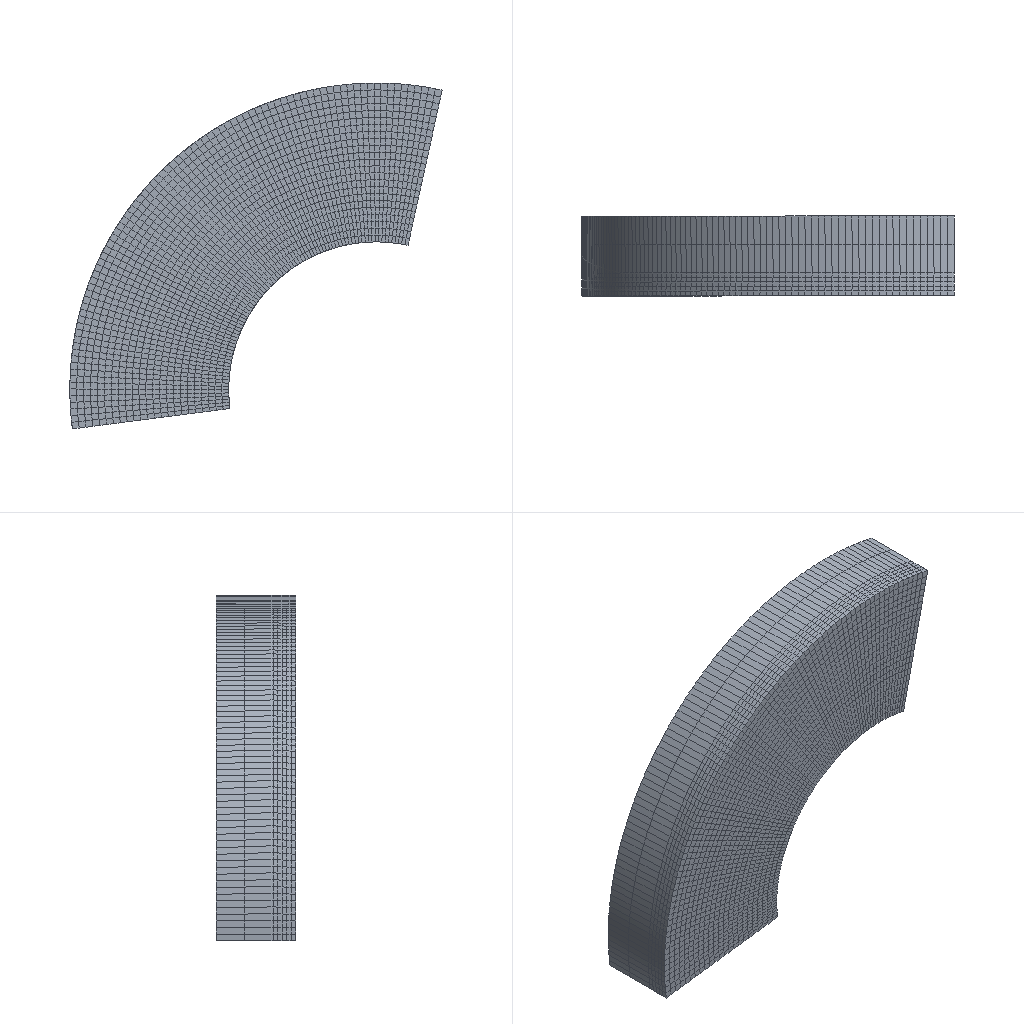Simulation study | abaqus
Set-up summary:
category,name,step,type,value,unit,region
solver,abaqus
solver,version,,,Abaqus/Explicit 2020
units,not stated in the deck,,not stated
analysis,deck,,transient,transient
load_step,Step-1,Step-1,transient,nlgeom=True
contact,interactions,,,general=0 pairs=1 ties=0
load_step,requested,,,1
mesh,nodes,,,17698
mesh,elements,,,14845
element_type,R3D3,,rigid,14
element_type,R3D4,,rigid,985
element_type,C3D8R,,solid,13846
load,load commands in deck,,count,1
bc,support commands in deck,,count,7
material,MATERIAL-1,,in results
check,setup vs results,,match,"per instance, exact: element labels, types and connectivity; labels of the nodes the elements use; coordinates of those nodes at SINGLE_PRECISION in 1 of 2 instance(s)"
Abaqus input file, long lists of numbers shortened:
*Heading
** Job name: Job-2 Model name: Model-1-Copy
** Generated by: Abaqus/CAE 2020
*Preprint, echo=NO, model=NO, history=NO, contact=NO
**
** PARTS
**
*Part, name=work
*Node
      1,  0.8032,          -5.,  -4.555
      2,  0.5209,  0.04385,  -2.954
** (992 more lines like these left out)
*Element, type=R3D4
1,   1,  15, 228,  19
2,  15,   2,   3, 228
** (983 more lines like these left out)
*Element, type=R3D3
77, 415, 376, 414
78, 365, 364, 321
** (12 more lines like these left out)
*End Part
**
*Part, name=work2
*Node
      1,   29.301,   24.684,          10.
      2,  -36.312,   49.078,          10.
** (16702 more lines like these left out)
*Element, type=C3D8R
   1,    1,   17,  675,  230,  444, 4585, 7355, 4415
   2,   17,   18,  676,  675, 4585, 4586, 7356, 7355
** (13844 more lines like these left out)
*Nset, nset=Set-1, generate
     1,  16704,      1
*Elset, elset=Set-1, generate
     1,  13846,      1
** Section: bing
*Solid Section, elset=Set-1, material=Material-1
,
*End Part
**
**
** ASSEMBLY
**
*Assembly, name=Assembly
**
*Instance, name=work-1, part=work
-40.107,           5., -16.132
-40.107,           5., -16.132, -40.126, 5.142, -17.122, 15.357
*End Instance
**
*Instance, name=work2-1, part=work2
0.00232,           0., 20.53
0.00232,           0., 20.53, -0.9849, 0.1125, 20.643, 90.734
*End Instance
**
*Node
      1,   87.459,          10.,  -1.747
*Nset, nset=Set-3, instance=work2-1
    5,    6,    7,    8,    9,   10,  231,  232,  233,  234,  235,  236,  237,  238,  239,  240
  241,  242,  243,  244,  245,  246,  247,  248,  249,  250,  251,  252,  253,  254,  255,  256
** (129 more lines like these left out)
*Elset, elset=Set-3, instance=work2-1, generate
 1979,  3956,     1
*Nset, nset=Set-7
 1,
*Nset, nset=b_Set-5, instance=work-1, generate
   1,  994,    1
*Elset, elset=b_Set-5, instance=work-1, generate
   1,  999,    1
*Nset, nset=s_Set-4, instance=work2-1
    1,    2,    3,    4,   11,   12,   13,   14,   15,   16,   17,   18,   19,   20,   21,   22
   23,   24,   25,   26,   27,   28,   29,   30,   31,   32,   33,   34,   35,   36,   37,   38
** (197 more lines like these left out)
*Elset, elset=s_Set-4, instance=work2-1
  3957,  3958,  3959,  3960,  3961,  3962,  3963,  3964,  3965,  3966,  3967,  3968,  3969,  3970,  3971,  3972
  3973,  3974,  3975,  3976,  3977,  3978,  3979,  3980,  3981,  3982,  3983,  3984,  3985,  3986,  3987,  3988
** (176 more lines like these left out)
*Nset, nset=s_Set-6, instance=work2-1
     1,     2,     3,     4,    11,    12,    13,    14,    15,    16,    17,    18,    19,    20,    21,    22
    23,    24,    25,    26,    27,    28,    29,    30,    31,    32,    33,    34,    35,    36,    37,    38
** (781 more lines like these left out)
*Elset, elset=s_Set-6, instance=work2-1, generate
  3957,  13846,      1
*Nset, nset=_PickedSet8, internal
 1,
*Elset, elset=_m_Surf-1_SPOS, internal, instance=work-1, generate
   1,  999,    1
*Surface, type=ELEMENT, name=m_Surf-1
_m_Surf-1_SPOS, SPOS
*Elset, elset=_m_Surf-2_SPOS, internal, instance=work-1, generate
   1,  999,    1
*Surface, type=ELEMENT, name=m_Surf-2
_m_Surf-2_SPOS, SPOS
*Surface, type=NODE, name=s_Set-6_CNS_, internal
s_Set-6, 1.
** Constraint: Constraint-1
*Rigid Body, ref node=_PickedSet8, elset=b_Set-5
*End Assembly
**
** MATERIALS
**
*Material, name=Material-1
*Damage Initiation, criterion=SHEAR
 1.1,0.,0.
*Damage Evolution, type=DISPLACEMENT
 0.05,
*Density
 9e-10,
*Elastic
10000., 0.3
*Plastic
 5.,   0.
10., 0.01
**
** INTERACTION PROPERTIES
**
*Surface Interaction, name=IntProp-1
*Friction
 0.14,
*Surface Behavior, pressure-overclosure=HARD
** ----------------------------------------------------------------
**
** STEP: Step-1
**
*Step, name=Step-1, nlgeom=YES
*Dynamic, Explicit
, 0.12
*Bulk Viscosity
0.06, 1.2
** Mass Scaling: Semi-Automatic
**               Whole Model
*Fixed Mass Scaling, factor=500.
**
** BOUNDARY CONDITIONS
**
** Name: BC-1 Type: 对称/反对称/完全固定
*Boundary
Set-3, ENCASTRE
** Name: [REDACTED] : Velocity/Angular velocity
*Boundary, type=VELOCITY
Set-7, 1, 1
Set-7, 2, 2
Set-7, 3, 3
Set-7, 4, 4
Set-7, 5, 5, 15.
Set-7, 6, 6
**
** INTERACTIONS
**
** Interaction: Int-1
*Contact Pair, interaction=IntProp-1, mechanical constraint=KINEMATIC, cpset=Int-1
m_Surf-2, s_Set-6_CNS_
**
** OUTPUT REQUESTS
**
*Restart, write, number interval=1, time marks=NO
**
** FIELD OUTPUT: F-Output-1
**
*Output, field, number interval=30
*Node Output
A, CF, RF, RM, RT, U, V
*Element Output, directions=YES
E, EVF, LE, MISES, MISESMAX, MISESONLY, NE, PE, PEEQ, PEEQMAX, PEEQT, PEEQVAVG, PEMAG, PEVAVG, PRESSONLY, S
SEQUT, SF, STATUS, SVAVG, YIELDPOT
*Contact Output
CDISP, CSTRESS
**
** HISTORY OUTPUT: H-Output-1
**
*Output, history, time interval=2.4e-06
*Node Output, nset=Set-7
RF1, RF2, RF3, RM1, RM2, RM3
*End Step
Results summary:
result,step,Step-1,completed,increments=25604 time=0.12/0.12
result,analysis,,,transient
result,last_loadstep,,,1
result,analysis steps,,count,1
result,primary field,,,U
result,reaction total,,FX,-2902.138,model units
result,reaction total,,FY,-113.985,model units
result,reaction total,,FZ,-3104.602,model units